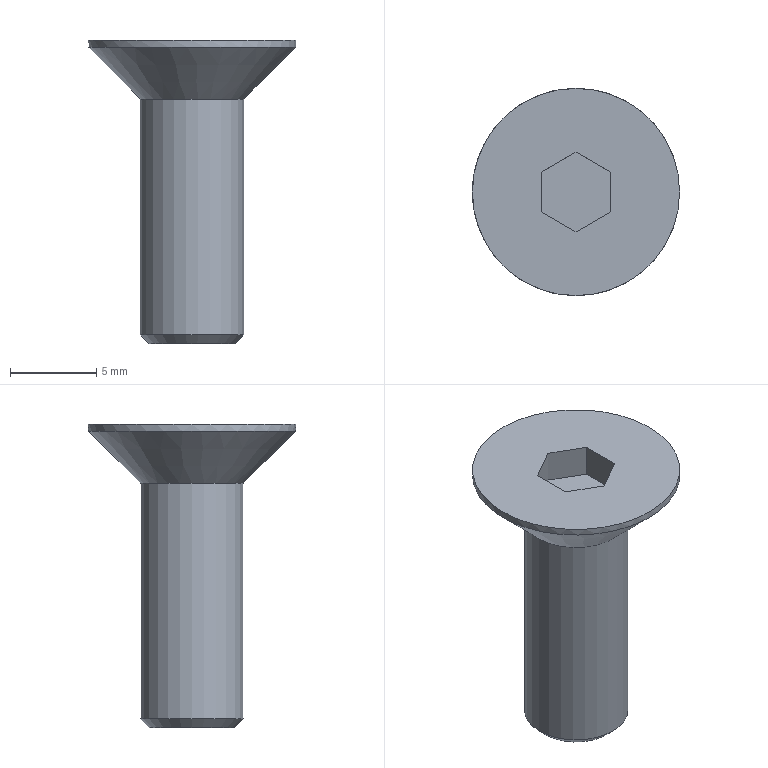Part | STEP file | solid 153 | 1 solid | 13 faces | box 12 x 12 x 17.55 mm | volume 614.689 mm3 | plane 9 | cone 2 | cylinder 2 | commonest cylinder face diameters 6 x1 12 x1